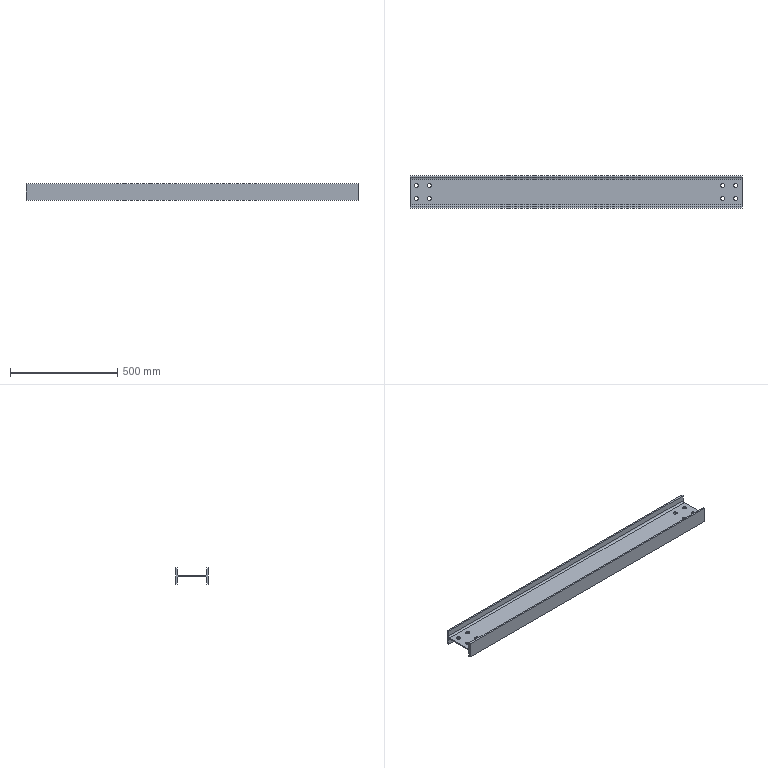Part | STEP file | 粉仓辅梁11主体_Default<As Machined> | 1 solid | 34 faces | box 1545 x 150 x 75 mm | volume 2746388 mm3 | cylinder 20 | plane 14 | commonest cylinder face diameters 19 x16 16 x4